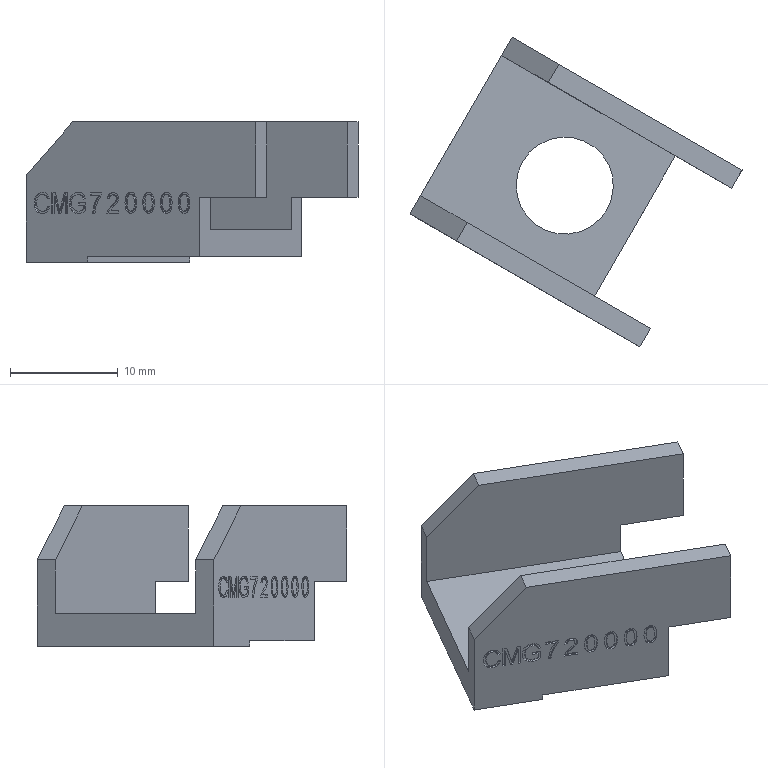Part | NX | features 18 2 | 1 solid | 87 faces | box 30.754 x 28.668 x 13 mm | volume 1621 mm3 | plane 61 | spline 24 | cylinder 2 | commonest cylinder face diameters 9 x2